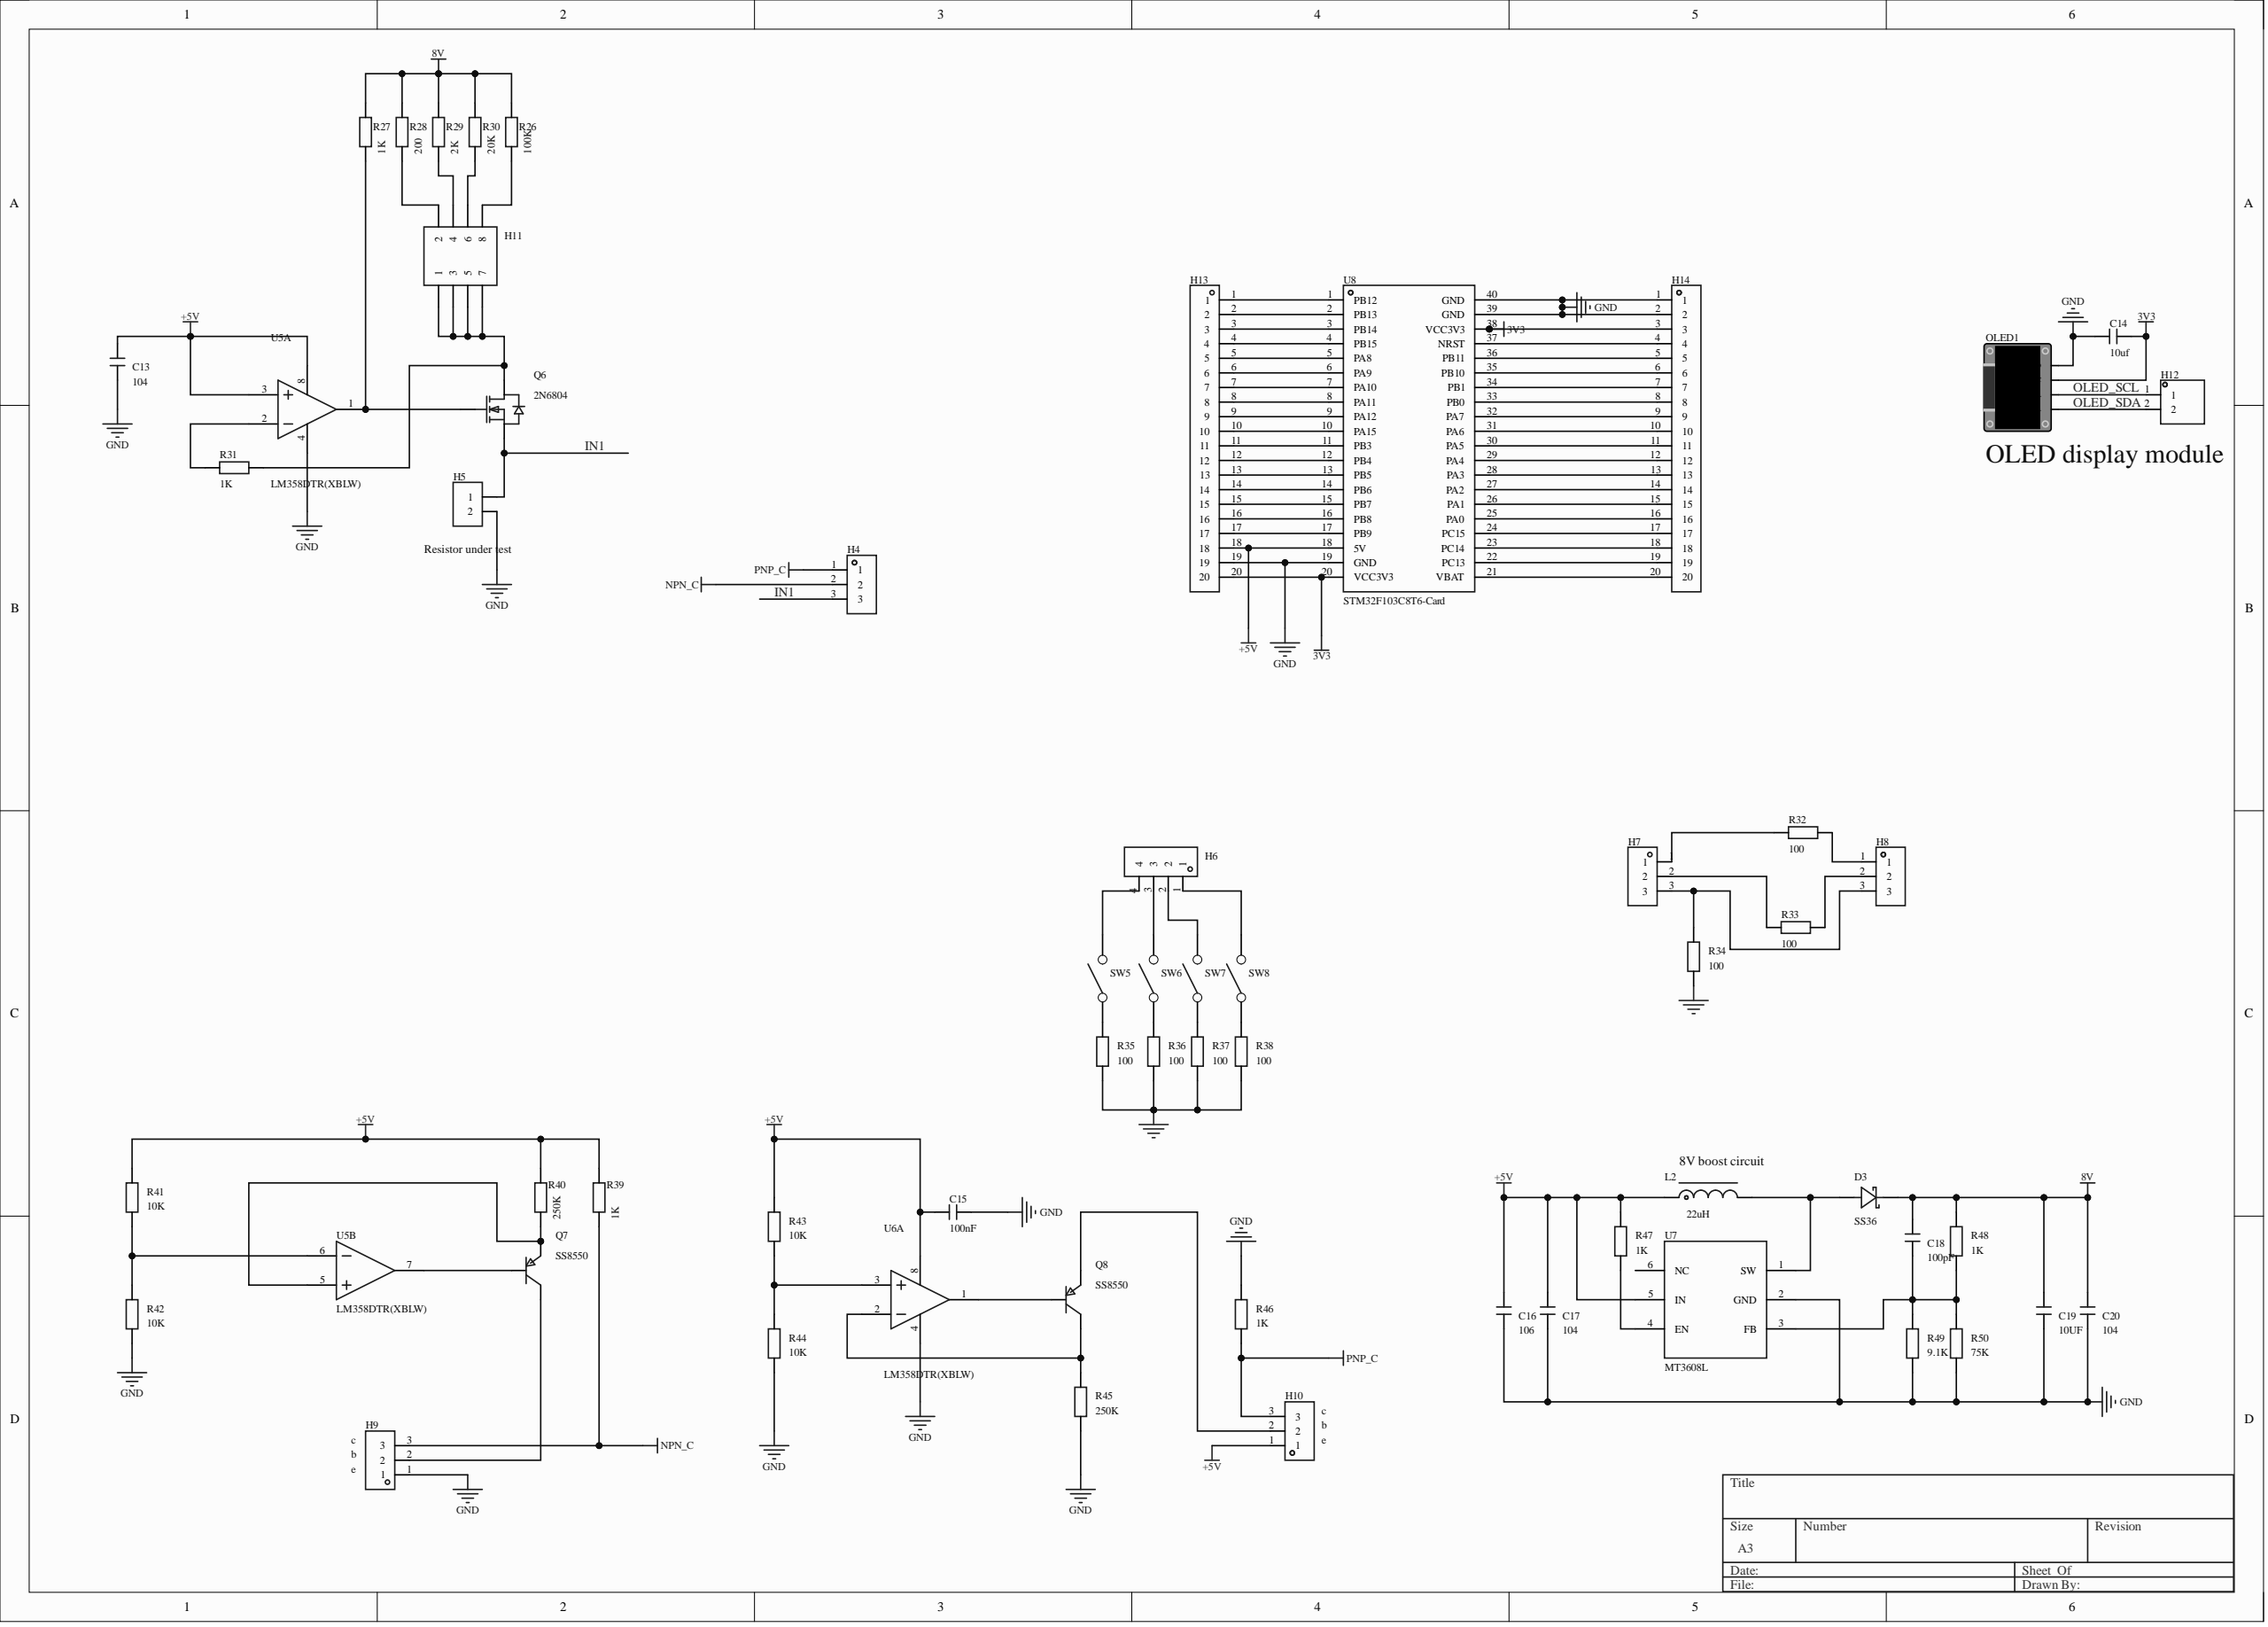Circuit board | Altium Designer | 58 parts | 73 nets
Bill of materials:
Comment,Description,Designator,Footprint,LibRef,Quantity
"104","","C13, C17, C20","C0603","CAP_0603","3"
"10uf","","C14, C19","C0603","CAP_0603","2"
"100nF","","C15","C0603","CAP_0603","1"
"106","","C16","C0603","CAP_0603","1"
"100pF","","C18","C0603","CAP_0603","1"
"SS36","Diode configuration: discrete; forward voltage drop (Vf): 700mV@3.0A; DC reverse voltage (Vr): 60V; rectifier current: 3A;","D3","SMA_L4.3-W2.6-LS5.0-FD","SS36_C7420367","1"
"","","H4, H7, H8, H9, H10","HDR-TH_3P-P2.54-V-F","HDR-F_2.54_1x3P","5"
"","","H5","HDR-TH_2P-P2.54-V-F","HDR-F_2.54_1x2P","1"
"","","H6","HDR-TH_4P-P2.54-V-M","HDR-M_2.54_1x4P","1"
"","","H11","HDR-TH_8P-P2.54-V-M-R2-C4-S2.54","HDR-M_2.54_2x4","1"
"","","H12","HDR-TH_2P-P2.54-V-M-1","HDR-M_2.54_1x2P","1"
"","Pitch: 2.54mm; total pin count: 20; rows: 1; pin structure: -; row spacing: -; mounting type: through-hole; round/square pin: -; rated current: -; rated voltage: -; mating pin length: -; plastic height: -; contact material: brass; contact plating: -; colour: black;","H13, H14","HDR-TH_20P-P2.54-V-M-1","HDR-M_2.54_1x20P","2"
"22uH","Inductance: 22uH; tolerance: ±20%; rated current: 3A;","L2","IND-SMD_L7.1-W6.6","YSPI0630A-220M","1"
"","","OLED1","0.96OLED_4P","0.96OLED模块_4P","1"
"2N6804","Type: 1 N-channel; drain-source voltage (Vdss): 55V; continuous drain current (Id): 49A; on-resistance (RDS(on)@Vgs,Id): 17.5mO@10V,25A; power (Pd): 94W; threshold voltage (Vgs(th)@Id): 4V@250uA;","Q6","TO-220-3_L10.0-W4.5-P2.54-L","IRFZ44NPBF","1"
"SS8550","Transistor type: PNP; collector current (Ic): 1.5A; collector-emitter breakdown voltage (Vceo): 25V; power (Pd): 300mW; DC current gain (hFE@Ic,Vce): 120@100mA,1.0V;","Q7, Q8","SOT-23-3_L2.9-W1.3-P1.90-LS2.4-BR","SS8550_C7420371","2"
"100K","","R26","R0603","Res_0603","1"
"1K","","R27, R31, R39, R46, R47, R48","R0603","Res_0603","6"
"200","","R28","R0603","Res_0603","1"
"2K","","R29","R0603","Res_0603","1"
"20K","","R30","R0603","Res_0603","1"
"100","","R32, R33, R34, R35, R36, R37, R38","R0603","Res_0603","7"
"250K","","R40, R45","R0603","Res_0603","2"
"10K","","R41, R42, R43, R44","R0603","Res_0603","4"
"9.1K","","R49","R0603","Res_0603","1"
"75K","","R50","R0603","Res_0603","1"
"TS-1088-AR02016","","SW5, SW6, SW7, SW8","SW-SMD_L3.9-W3.0-P4.45","TS-1088-AR02016","4"
"LM358DTR(XBLW)","Amplifier count: dual; gain-bandwidth product (GBP): 1MHz; input bias current (Ib): 45nA; input offset voltage (Vos): 7mV;","U5, U6","SOIC-8_L4.9-W4.0-P1.27-LS6.0-BL","LM358DTR(XBLW)","2"
"MT3608L","Operating voltage: 2.2V~16V; output current: 2.5A;","U7","SOT-23-6_L2.9-W1.6-P0.95-LS2.8-BL_3","MT3608L","1"
"STM32F103C8T6-Card","","U8","CONN-TH_L53.3-W22.9_STM32F103C8T6-CARD","STM32F103C8T6-Card","1"
Netlist (Protel format):
[
C13
C0603
104



]
[
C14
C0603
10uf



]
[
C15
C0603
100nF



]
[
C16
C0603
106



]
[
C17
C0603
104



]
[
C18
C0603
100pF



]
[
C19
C0603
10UF



]
[
C20
C0603
104



]
[
D3
SMA_L4.3-W2.6-LS5.0-FD
SS36



]
[
H4
HDR-TH_3P-P2.54-V-F




]
[
H5
HDR-TH_2P-P2.54-V-F




]
[
H6
HDR-TH_4P-P2.54-V-M




]
[
H7
HDR-TH_3P-P2.54-V-F




]
[
H8
HDR-TH_3P-P2.54-V-F




]
[
H9
HDR-TH_3P-P2.54-V-F




]
[
H10
HDR-TH_3P-P2.54-V-F




]
[
H11
HDR-TH_8P-P2.54-V-M-R2-C4-S2.54




]
[
H12
HDR-TH_2P-P2.54-V-M-1




]
[
H13
HDR-TH_20P-P2.54-V-M-1




]
[
H14
HDR-TH_20P-P2.54-V-M-1




]
[
L2
IND-SMD_L7.1-W6.6
22uH



]
[
OLED1
0.96OLED_4P




]
[
Q6
TO-220-3_L10.0-W4.5-P2.54-L
2N6804



]
[
Q7
SOT-23-3_L2.9-W1.3-P1.90-LS2.4-BR
SS8550



]
[
Q8
SOT-23-3_L2.9-W1.3-P1.90-LS2.4-BR
SS8550



]
[
R26
R0603
100K



]
[
R27
R0603
1K



]
[
R28
R0603
200



]
[
R29
R0603
2K



]
[
R30
R0603
20K



]
[
R31
R0603
1K



]
[
R32
R0603
100



]
[
R33
R0603
100



]
[
R34
R0603
100



]
[
R35
R0603
100



]
[
R36
R0603
100



]
[
R37
R0603
100



]
[
R38
R0603
100



]
[
R39
R0603
1K



]
[
R40
R0603
250K



]
[
R41
R0603
10K



]
[
R42
R0603
10K



]
[
R43
R0603
10K



]
[
R44
R0603
10K



]
[
R45
R0603
250K



]
[
R46
R0603
1K



]
[
R47
R0603
1K



]
[
R48
R0603
1K



]
[
R49
R0603
9.1K



]
[
R50
R0603
75K



]
[
SW5
SW-SMD_L3.9-W3.0-P4.45
TS-1088-AR02016



]
[
SW6
SW-SMD_L3.9-W3.0-P4.45
TS-1088-AR02016



]
[
SW7
SW-SMD_L3.9-W3.0-P4.45
TS-1088-AR02016



]
[
SW8
SW-SMD_L3.9-W3.0-P4.45
TS-1088-AR02016



]
[
U5
SOIC-8_L4.9-W4.0-P1.27-LS6.0-BL
LM358DTR(XBLW)



]
[
U6
SOIC-8_L4.9-W4.0-P1.27-LS6.0-BL
LM358DTR(XBLW)



]
[
U7
SOT-23-6_L2.9-W1.6-P0.95-LS2.8-BL_3
MT3608L



]
[
U8
CONN-TH_L53.3-W22.9_STM32F103C8T6-CARD
STM32F103C8T6-Card



]
(
OLED_SDA
H12-2
OLED1-4
)
(
OLED_SCL
H12-1
OLED1-3
)
(
NetR47_1
R47-1
U7-4
)
(
NetR43_1
R43-1
R44-2
U6-3
)
(
NetR41_1
R41-1
R42-2
U5-6
)
(
NetR38_1
R38-1
SW8-1
)
(
NetR37_1
R37-1
SW7-1
)
(
NetR36_1
R36-1
SW6-1
)
(
NetR35_1
R35-1
SW5-1
)
(
NetR31_2
R31-2
U5-2
)
(
NetQ8_3
Q8-3
R45-2
U6-2
)
(
NetQ8_1
Q8-1
U6-1
)
(
NetQ7_2
Q7-2
R40-1
U5-5
)
(
NetQ7_1
Q7-1
U5-7
)
(
NetQ6_1
Q6-1
R27-1
U5-1
)
(
NetH14_20
H14-20
U8-21
)
(
NetH14_19
H14-19
U8-22
)
(
NetH14_18
H14-18
U8-23
)
(
NetH14_17
H14-17
U8-24
)
(
NetH14_16
H14-16
U8-25
)
(
NetH14_15
H14-15
U8-26
)
(
NetH14_14
H14-14
U8-27
)
(
NetH14_13
H14-13
U8-28
)
(
NetH14_12
H14-12
U8-29
)
(
NetH14_11
H14-11
U8-30
)
(
NetH14_10
H14-10
U8-31
)
(
NetH14_9
H14-9
U8-32
)
(
NetH14_8
H14-8
U8-33
)
(
NetH14_7
H14-7
U8-34
)
(
NetH14_6
H14-6
U8-35
)
(
NetH14_5
H14-5
U8-36
)
(
NetH14_4
H14-4
U8-37
)
(
NetH13_17
H13-17
U8-17
)
(
NetH13_16
H13-16
U8-16
)
(
NetH13_15
H13-15
U8-15
)
(
NetH13_14
H13-14
U8-14
)
(
NetH13_13
H13-13
U8-13
)
(
NetH13_12
H13-12
U8-12
)
(
NetH13_11
H13-11
U8-11
)
(
NetH13_10
H13-10
U8-10
)
(
NetH13_9
H13-9
U8-9
)
(
NetH13_8
H13-8
U8-8
)
(
NetH13_7
H13-7
U8-7
)
(
NetH13_6
H13-6
U8-6
)
(
NetH13_5
H13-5
U8-5
)
(
NetH13_4
H13-4
U8-4
)
(
NetH13_3
H13-3
U8-3
)
(
NetH13_2
H13-2
U8-2
)
(
NetH13_1
H13-1
U8-1
)
(
NetH11_8
H11-8
R26-1
)
(
NetH11_6
H11-6
R30-1
)
(
NetH11_4
H11-4
R29-1
)
(
NetH11_2
H11-2
R28-1
)
(
NetH11_1
H11-1
H11-3
H11-5
H11-7
Q6-2
R31-1
)
(
NetH10_2
H10-2
Q8-2
)
(
NetH9_2
H9-2
Q7-3
)
(
NetH8_2
H8-2
R33-1
)
(
NetH8_1
H8-1
R32-1
)
(
NetH7_3
H7-3
H8-3
R34-1
)
(
NetH7_2
H7-2
R33-2
)
(
NetH7_1
H7-1
R32-2
)
(
NetH6_4
H6-4
SW5-2
)
(
NetH6_3
H6-3
SW6-2
)
(
NetH6_2
H6-2
SW7-2
)
(
NetH6_1
H6-1
SW8-2
)
(
NetD3_1
D3-1
L2-2
U7-1
)
(
NetC18_2
C18-2
R48-2
R49-2
R50-2
U7-3
)
(
IN1
H4-3
H5-1
Q6-3
)
(
C
H4-1
H4-2
H9-3
H10-3
R39-1
R46-1
)
(
+5V
C13-2
C15-2
C16-1
C17-1
H10-1
H13-18
L2-1
R39-2
R40-2
R41-2
R43-2
R47-2
U5-3
U5-8
U6-8
U7-5
U8-18
)
(
8V
C18-1
C19-1
C20-1
D3-2
R26-2
R27-2
R28-2
R29-2
R30-2
R48-1
)
(
5V
C13-1
C14-2
C15-1
C16-2
C17-2
C19-2
C20-2
H5-2
H9-1
H13-19
H14-1
H14-2
OLED1-1
R34-2
R35-2
R36-2
R37-2
R38-2
R42-1
R44-1
R45-1
R46-2
R49-1
R50-1
U5-4
U6-4
U7-2
U8-19
U8-39
U8-40
)
(
3V3
C14-1
H13-20
H14-3
OLED1-2
U8-20
U8-38
)